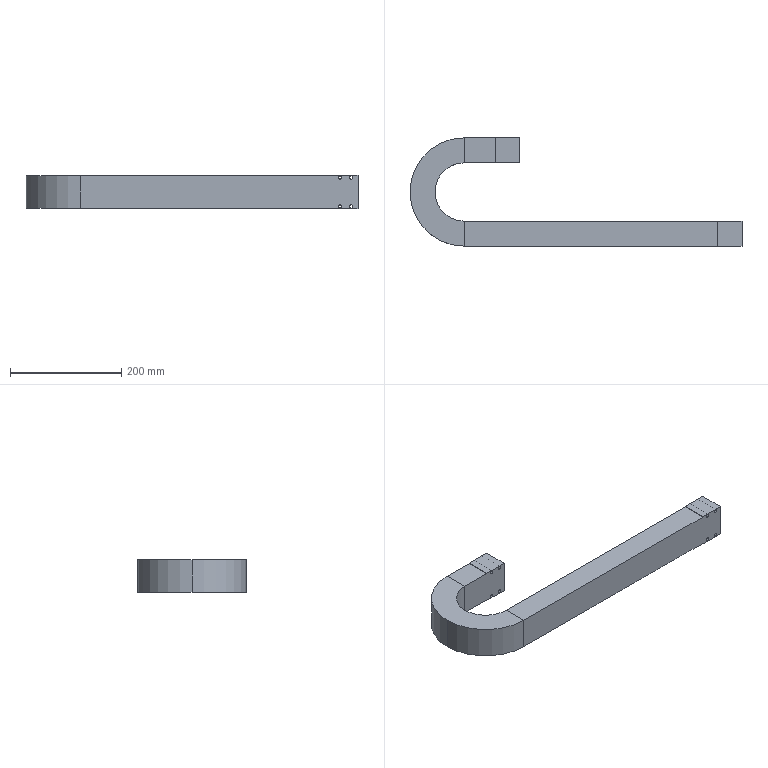Part | STEP file | Drag chain 3038 | 1 solid | 40 faces | box 597.5 x 195 x 60 mm | volume 2179375 mm3 | cylinder 20 | plane 20 | commonest cylinder face diameters 5.8 x16 105 x2 195 x2